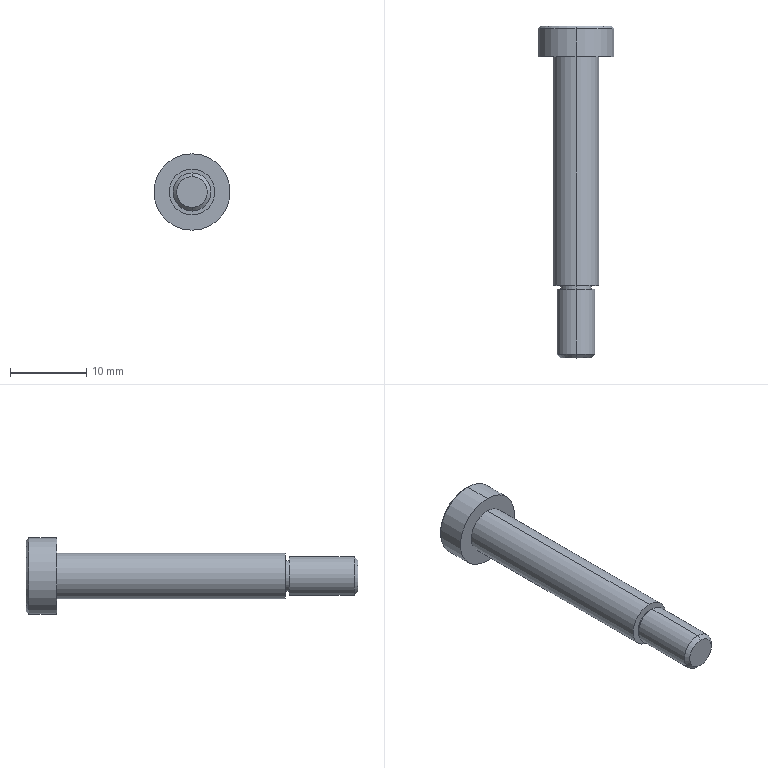Part | SolidWorks | features BaseBody 1, MoveFace 1 | 1 solid | 24 faces | box 10 x 43.5 x 10 mm | volume 1326 mm3 | plane 12 | cylinder 8 | cone 4 | commonest cylinder face diameters 4 x2 5 x2 6 x2 10 x2
STEP:
#1=CARTESIAN_POINT('',(0.,-8.5,3.));
#2=VERTEX_POINT('',#1);
#3=CARTESIAN_POINT('',(0.,-8.5,-3.));
#4=VERTEX_POINT('',#3);
#5=CARTESIAN_POINT('',(0.,-8.5,0.));
#6=DIRECTION('',(0.,1.,0.));
#7=DIRECTION('',(0.,0.,1.));
#8=AXIS2_PLACEMENT_3D('',#5,#6,#7);
#9=CIRCLE('',#8,3.);
#10=EDGE_CURVE('',#2,#4,#9,.T.);
#11=ORIENTED_EDGE('',*,*,#10,.T.);
#12=CARTESIAN_POINT('',(0.,21.5,-3.));
#13=VERTEX_POINT('',#12);
#14=CARTESIAN_POINT('',(0.,0.,-3.));
#15=DIRECTION('',(0.,1.,0.));
#16=VECTOR('',#15,1000.);
#17=LINE('',#14,#16);
#18=EDGE_CURVE('',#4,#13,#17,.T.);
#19=ORIENTED_EDGE('',*,*,#18,.T.);
#20=CARTESIAN_POINT('',(0.,21.5,3.));
#21=VERTEX_POINT('',#20);
#22=CARTESIAN_POINT('',(0.,21.5,0.));
#23=DIRECTION('',(0.,-1.,0.));
#24=DIRECTION('',(0.,0.,1.));
#25=AXIS2_PLACEMENT_3D('',#22,#23,#24);
#26=CIRCLE('',#25,3.);
#27=EDGE_CURVE('',#13,#21,#26,.T.);
#28=ORIENTED_EDGE('',*,*,#27,.T.);
#29=CARTESIAN_POINT('',(0.,0.,3.));
#30=DIRECTION('',(0.,1.,0.));
#31=VECTOR('',#30,1000.);
#32=LINE('',#29,#31);
#33=EDGE_CURVE('',#2,#21,#32,.T.);
#34=ORIENTED_EDGE('',*,*,#33,.F.);
#35=EDGE_LOOP('',(#11,#19,#28,#34));
#36=FACE_OUTER_BOUND('',#35,.T.);
#37=CARTESIAN_POINT('',(0.,0.,0.));
#38=DIRECTION('',(0.,1.,0.));
#39=DIRECTION('',(0.,0.,1.));
#40=AXIS2_PLACEMENT_3D('',#37,#38,#39);
#41=CYLINDRICAL_SURFACE('',#40,3.);
#42=ADVANCED_FACE('',(#36),#41,.T.);
#43=CARTESIAN_POINT('',(0.,21.5,5.));
#44=VERTEX_POINT('',#43);
#45=CARTESIAN_POINT('',(0.,21.5,-5.));
#46=VERTEX_POINT('',#45);
#47=CARTESIAN_POINT('',(0.,21.5,0.));
#48=DIRECTION('',(0.,1.,0.));
#49=DIRECTION('',(0.,0.,1.));
#50=AXIS2_PLACEMENT_3D('',#47,#48,#49);
#51=CIRCLE('',#50,5.);
#52=EDGE_CURVE('',#44,#46,#51,.T.);
#53=ORIENTED_EDGE('',*,*,#52,.T.);
#54=CARTESIAN_POINT('',(0.,25.167,-5.));
#55=VERTEX_POINT('',#54);
#56=CARTESIAN_POINT('',(0.,0.,-5.));
#57=DIRECTION('',(0.,1.,0.));
#58=VECTOR('',#57,1000.);
#59=LINE('',#56,#58);
#60=EDGE_CURVE('',#46,#55,#59,.T.);
#61=ORIENTED_EDGE('',*,*,#60,.T.);
#62=CARTESIAN_POINT('',(0.,25.167,5.));
#63=VERTEX_POINT('',#62);
#64=CARTESIAN_POINT('',(0.,25.167,0.));
#65=DIRECTION('',(0.,-1.,0.));
#66=DIRECTION('',(0.,0.,1.));
#67=AXIS2_PLACEMENT_3D('',#64,#65,#66);
#68=CIRCLE('',#67,5.);
#69=EDGE_CURVE('',#55,#63,#68,.T.);
#70=ORIENTED_EDGE('',*,*,#69,.T.);
#71=CARTESIAN_POINT('',(0.,0.,5.));
#72=DIRECTION('',(0.,1.,0.));
#73=VECTOR('',#72,1000.);
#74=LINE('',#71,#73);
#75=EDGE_CURVE('',#44,#63,#74,.T.);
#76=ORIENTED_EDGE('',*,*,#75,.F.);
#77=EDGE_LOOP('',(#53,#61,#70,#76));
#78=FACE_OUTER_BOUND('',#77,.T.);
#79=CARTESIAN_POINT('',(0.,0.,0.));
#80=DIRECTION('',(0.,1.,0.));
#81=DIRECTION('',(0.,0.,1.));
#82=AXIS2_PLACEMENT_3D('',#79,#80,#81);
#83=CYLINDRICAL_SURFACE('',#82,5.);
#84=ADVANCED_FACE('',(#78),#83,.T.);
#85=CARTESIAN_POINT('',(0.,-9.,2.));
#86=VERTEX_POINT('',#85);
#87=CARTESIAN_POINT('',(0.,-9.,-2.));
#88=VERTEX_POINT('',#87);
#89=CARTESIAN_POINT('',(0.,-9.,0.));
#90=DIRECTION('',(0.,1.,0.));
#91=DIRECTION('',(0.,0.,1.));
#92=AXIS2_PLACEMENT_3D('',#89,#90,#91);
#93=CIRCLE('',#92,2.);
#94=EDGE_CURVE('',#86,#88,#93,.T.);
#95=ORIENTED_EDGE('',*,*,#94,.T.);
#96=CARTESIAN_POINT('',(0.,-8.5,-2.));
#97=VERTEX_POINT('',#96);
#98=CARTESIAN_POINT('',(0.,-18.,-2.));
#99=DIRECTION('',(0.,1.,0.));
#100=VECTOR('',#99,1000.);
#101=LINE('',#98,#100);
#102=EDGE_CURVE('',#88,#97,#101,.T.);
#103=ORIENTED_EDGE('',*,*,#102,.T.);
#104=CARTESIAN_POINT('',(0.,-8.5,2.));
#105=VERTEX_POINT('',#104);
#106=CARTESIAN_POINT('',(0.,-8.5,0.));
#107=DIRECTION('',(0.,-1.,0.));
#108=DIRECTION('',(0.,0.,1.));
#109=AXIS2_PLACEMENT_3D('',#106,#107,#108);
#110=CIRCLE('',#109,2.);
#111=EDGE_CURVE('',#97,#105,#110,.T.);
#112=ORIENTED_EDGE('',*,*,#111,.T.);
#113=CARTESIAN_POINT('',(0.,-18.,2.));
#114=DIRECTION('',(0.,1.,0.));
#115=VECTOR('',#114,1000.);
#116=LINE('',#113,#115);
#117=EDGE_CURVE('',#86,#105,#116,.T.);
#118=ORIENTED_EDGE('',*,*,#117,.F.);
#119=EDGE_LOOP('',(#95,#103,#112,#118));
#120=FACE_OUTER_BOUND('',#119,.T.);
#121=CARTESIAN_POINT('',(0.,-18.,0.));
#122=DIRECTION('',(0.,1.,0.));
#123=DIRECTION('',(0.,0.,1.));
#124=AXIS2_PLACEMENT_3D('',#121,#122,#123);
#125=CYLINDRICAL_SURFACE('',#124,2.);
#126=ADVANCED_FACE('',(#120),#125,.T.);
#127=CARTESIAN_POINT('',(0.,25.5,-4.667));
#128=VERTEX_POINT('',#127);
#129=CARTESIAN_POINT('',(0.,25.5,4.667));
#130=VERTEX_POINT('',#129);
#131=CARTESIAN_POINT('',(0.,25.5,0.));
#132=DIRECTION('',(0.,-1.,0.));
#133=DIRECTION('',(0.,0.,-1.));
#134=AXIS2_PLACEMENT_3D('',#131,#132,#133);
#135=CIRCLE('',#134,4.667);
#136=EDGE_CURVE('',#128,#130,#135,.T.);
#137=ORIENTED_EDGE('',*,*,#136,.T.);
#138=CARTESIAN_POINT('',(0.,25.167,5.));
#139=DIRECTION('',(0.,-0.7071,0.7071));
#140=VECTOR('',#139,1000.);
#141=LINE('',#138,#140);
#142=EDGE_CURVE('',#130,#63,#141,.T.);
#143=ORIENTED_EDGE('',*,*,#142,.T.);
#144=ORIENTED_EDGE('',*,*,#69,.F.);
#145=CARTESIAN_POINT('',(0.,25.167,-5.));
#146=DIRECTION('',(0.,-0.7071,-0.7071));
#147=VECTOR('',#146,1000.);
#148=LINE('',#145,#147);
#149=EDGE_CURVE('',#128,#55,#148,.T.);
#150=ORIENTED_EDGE('',*,*,#149,.F.);
#151=EDGE_LOOP('',(#137,#143,#144,#150));
#152=FACE_OUTER_BOUND('',#151,.T.);
#153=CARTESIAN_POINT('',(0.,25.167,0.));
#154=DIRECTION('',(0.,-1.,0.));
#155=DIRECTION('',(0.,0.,-1.));
#156=AXIS2_PLACEMENT_3D('',#153,#154,#155);
#157=CONICAL_SURFACE('',#156,5.,0.7854);
#158=ADVANCED_FACE('',(#152),#157,.T.);
#159=CARTESIAN_POINT('',(0.,-17.509,2.5));
#160=VERTEX_POINT('',#159);
#161=CARTESIAN_POINT('',(0.,-17.509,-2.5));
#162=VERTEX_POINT('',#161);
#163=CARTESIAN_POINT('',(0.,-17.509,0.));
#164=DIRECTION('',(0.,1.,0.));
#165=DIRECTION('',(0.,0.,1.));
#166=AXIS2_PLACEMENT_3D('',#163,#164,#165);
#167=CIRCLE('',#166,2.5);
#168=EDGE_CURVE('',#160,#162,#167,.T.);
#169=ORIENTED_EDGE('',*,*,#168,.T.);
#170=CARTESIAN_POINT('',(0.,-9.,-2.5));
#171=VERTEX_POINT('',#170);
#172=CARTESIAN_POINT('',(0.,-18.,-2.5));
#173=DIRECTION('',(0.,1.,0.));
#174=VECTOR('',#173,1000.);
#175=LINE('',#172,#174);
#176=EDGE_CURVE('',#162,#171,#175,.T.);
#177=ORIENTED_EDGE('',*,*,#176,.T.);
#178=CARTESIAN_POINT('',(0.,-9.,2.5));
#179=VERTEX_POINT('',#178);
#180=CARTESIAN_POINT('',(0.,-9.,0.));
#181=DIRECTION('',(0.,-1.,0.));
#182=DIRECTION('',(0.,0.,1.));
#183=AXIS2_PLACEMENT_3D('',#180,#181,#182);
#184=CIRCLE('',#183,2.5);
#185=EDGE_CURVE('',#171,#179,#184,.T.);
#186=ORIENTED_EDGE('',*,*,#185,.T.);
#187=CARTESIAN_POINT('',(0.,-18.,2.5));
#188=DIRECTION('',(0.,1.,0.));
#189=VECTOR('',#188,1000.);
#190=LINE('',#187,#189);
#191=EDGE_CURVE('',#160,#179,#190,.T.);
#192=ORIENTED_EDGE('',*,*,#191,.F.);
#193=EDGE_LOOP('',(#169,#177,#186,#192));
#194=FACE_OUTER_BOUND('',#193,.T.);
#195=CARTESIAN_POINT('',(0.,-18.,0.));
#196=DIRECTION('',(0.,1.,0.));
#197=DIRECTION('',(0.,0.,1.));
#198=AXIS2_PLACEMENT_3D('',#195,#196,#197);
#199=CYLINDRICAL_SURFACE('',#198,2.5);
#200=ADVANCED_FACE('',(#194),#199,.T.);
#201=CARTESIAN_POINT('',(0.,-18.,2.009));
#202=VERTEX_POINT('',#201);
#203=CARTESIAN_POINT('',(0.,-18.,-2.009));
#204=VERTEX_POINT('',#203);
#205=CARTESIAN_POINT('',(0.,-18.,0.));
#206=DIRECTION('',(0.,1.,0.));
#207=DIRECTION('',(0.,0.,1.));
#208=AXIS2_PLACEMENT_3D('',#205,#206,#207);
#209=CIRCLE('',#208,2.009);
#210=EDGE_CURVE('',#202,#204,#209,.T.);
#211=ORIENTED_EDGE('',*,*,#210,.T.);
#212=CARTESIAN_POINT('',(0.,-17.509,-2.5));
#213=DIRECTION('',(0.,0.7071,-0.7071));
#214=VECTOR('',#213,1000.);
#215=LINE('',#212,#214);
#216=EDGE_CURVE('',#204,#162,#215,.T.);
#217=ORIENTED_EDGE('',*,*,#216,.T.);
#218=ORIENTED_EDGE('',*,*,#168,.F.);
#219=CARTESIAN_POINT('',(0.,-17.509,2.5));
#220=DIRECTION('',(0.,0.7071,0.7071));
#221=VECTOR('',#220,1000.);
#222=LINE('',#219,#221);
#223=EDGE_CURVE('',#202,#160,#222,.T.);
#224=ORIENTED_EDGE('',*,*,#223,.F.);
#225=EDGE_LOOP('',(#211,#217,#218,#224));
#226=FACE_OUTER_BOUND('',#225,.T.);
#227=CARTESIAN_POINT('',(0.,-17.509,0.));
#228=DIRECTION('',(0.,1.,0.));
#229=DIRECTION('',(0.,0.,1.));
#230=AXIS2_PLACEMENT_3D('',#227,#228,#229);
#231=CONICAL_SURFACE('',#230,2.5,0.7854);
#232=ADVANCED_FACE('',(#226),#231,.T.);
#233=ORIENTED_EDGE('',*,*,#18,.F.);
#234=CARTESIAN_POINT('',(0.,-8.5,0.));
#235=DIRECTION('',(0.,1.,0.));
#236=DIRECTION('',(0.,0.,1.));
#237=AXIS2_PLACEMENT_3D('',#234,#235,#236);
#238=CIRCLE('',#237,3.);
#239=EDGE_CURVE('',#4,#2,#238,.T.);
#240=ORIENTED_EDGE('',*,*,#239,.T.);
#241=ORIENTED_EDGE('',*,*,#33,.T.);
#242=CARTESIAN_POINT('',(0.,21.5,0.));
#243=DIRECTION('',(0.,-1.,0.));
#244=DIRECTION('',(0.,0.,1.));
#245=AXIS2_PLACEMENT_3D('',#242,#243,#244);
#246=CIRCLE('',#245,3.);
#247=EDGE_CURVE('',#21,#13,#246,.T.);
#248=ORIENTED_EDGE('',*,*,#247,.T.);
#249=EDGE_LOOP('',(#233,#240,#241,#248));
#250=FACE_OUTER_BOUND('',#249,.T.);
#251=CARTESIAN_POINT('',(0.,0.,0.));
#252=DIRECTION('',(0.,1.,0.));
#253=DIRECTION('',(0.,0.,1.));
#254=AXIS2_PLACEMENT_3D('',#251,#252,#253);
#255=CYLINDRICAL_SURFACE('',#254,3.);
#256=ADVANCED_FACE('',(#250),#255,.T.);
#257=ORIENTED_EDGE('',*,*,#52,.F.);
#258=CARTESIAN_POINT('',(0.,21.5,0.));
#259=DIRECTION('',(0.,1.,0.));
#260=DIRECTION('',(0.,0.,1.));
#261=AXIS2_PLACEMENT_3D('',#258,#259,#260);
#262=CIRCLE('',#261,5.);
#263=EDGE_CURVE('',#46,#44,#262,.T.);
#264=ORIENTED_EDGE('',*,*,#263,.F.);
#265=EDGE_LOOP('',(#257,#264));
#266=FACE_OUTER_BOUND('',#265,.T.);
#267=ORIENTED_EDGE('',*,*,#247,.F.);
#268=ORIENTED_EDGE('',*,*,#27,.F.);
#269=EDGE_LOOP('',(#267,#268));
#270=FACE_BOUND('',#269,.T.);
#271=CARTESIAN_POINT('',(5.,21.5,0.));
#272=DIRECTION('',(0.,1.,0.));
#273=DIRECTION('',(0.,0.,1.));
#274=AXIS2_PLACEMENT_3D('',#271,#272,#273);
#275=PLANE('',#274);
#276=ADVANCED_FACE('',(#266,#270),#275,.F.);
#277=ORIENTED_EDGE('',*,*,#10,.F.);
#278=ORIENTED_EDGE('',*,*,#239,.F.);
#279=EDGE_LOOP('',(#277,#278));
#280=FACE_OUTER_BOUND('',#279,.T.);
#281=CARTESIAN_POINT('',(0.,-8.5,0.));
#282=DIRECTION('',(0.,-1.,0.));
#283=DIRECTION('',(0.,0.,1.));
#284=AXIS2_PLACEMENT_3D('',#281,#282,#283);
#285=CIRCLE('',#284,2.);
#286=EDGE_CURVE('',#105,#97,#285,.T.);
#287=ORIENTED_EDGE('',*,*,#286,.F.);
#288=ORIENTED_EDGE('',*,*,#111,.F.);
#289=EDGE_LOOP('',(#287,#288));
#290=FACE_BOUND('',#289,.T.);
#291=CARTESIAN_POINT('',(3.,-8.5,0.));
#292=DIRECTION('',(0.,1.,0.));
#293=DIRECTION('',(0.,0.,1.));
#294=AXIS2_PLACEMENT_3D('',#291,#292,#293);
#295=PLANE('',#294);
#296=ADVANCED_FACE('',(#280,#290),#295,.F.);
#297=ORIENTED_EDGE('',*,*,#60,.F.);
#298=ORIENTED_EDGE('',*,*,#263,.T.);
#299=ORIENTED_EDGE('',*,*,#75,.T.);
#300=CARTESIAN_POINT('',(0.,25.167,0.));
#301=DIRECTION('',(0.,-1.,0.));
#302=DIRECTION('',(0.,0.,1.));
#303=AXIS2_PLACEMENT_3D('',#300,#301,#302);
#304=CIRCLE('',#303,5.);
#305=EDGE_CURVE('',#63,#55,#304,.T.);
#306=ORIENTED_EDGE('',*,*,#305,.T.);
#307=EDGE_LOOP('',(#297,#298,#299,#306));
#308=FACE_OUTER_BOUND('',#307,.T.);
#309=CARTESIAN_POINT('',(0.,0.,0.));
#310=DIRECTION('',(0.,1.,0.));
#311=DIRECTION('',(0.,0.,1.));
#312=AXIS2_PLACEMENT_3D('',#309,#310,#311);
#313=CYLINDRICAL_SURFACE('',#312,5.);
#314=ADVANCED_FACE('',(#308),#313,.T.);
#315=ORIENTED_EDGE('',*,*,#102,.F.);
#316=CARTESIAN_POINT('',(0.,-9.,0.));
#317=DIRECTION('',(0.,1.,0.));
#318=DIRECTION('',(0.,0.,1.));
#319=AXIS2_PLACEMENT_3D('',#316,#317,#318);
#320=CIRCLE('',#319,2.);
#321=EDGE_CURVE('',#88,#86,#320,.T.);
#322=ORIENTED_EDGE('',*,*,#321,.T.);
#323=ORIENTED_EDGE('',*,*,#117,.T.);
#324=ORIENTED_EDGE('',*,*,#286,.T.);
#325=EDGE_LOOP('',(#315,#322,#323,#324));
#326=FACE_OUTER_BOUND('',#325,.T.);
#327=CARTESIAN_POINT('',(0.,-18.,0.));
#328=DIRECTION('',(0.,1.,0.));
#329=DIRECTION('',(0.,0.,1.));
#330=AXIS2_PLACEMENT_3D('',#327,#328,#329);
#331=CYLINDRICAL_SURFACE('',#330,2.);
#332=ADVANCED_FACE('',(#326),#331,.T.);
#333=ORIENTED_EDGE('',*,*,#142,.F.);
#334=CARTESIAN_POINT('',(0.,25.5,0.));
#335=DIRECTION('',(0.,-1.,0.));
#336=DIRECTION('',(0.,0.,-1.));
#337=AXIS2_PLACEMENT_3D('',#334,#335,#336);
#338=CIRCLE('',#337,4.667);
#339=EDGE_CURVE('',#130,#128,#338,.T.);
#340=ORIENTED_EDGE('',*,*,#339,.T.);
#341=ORIENTED_EDGE('',*,*,#149,.T.);
#342=ORIENTED_EDGE('',*,*,#305,.F.);
#343=EDGE_LOOP('',(#333,#340,#341,#342));
#344=FACE_OUTER_BOUND('',#343,.T.);
#345=CARTESIAN_POINT('',(0.,25.167,0.));
#346=DIRECTION('',(0.,-1.,0.));
#347=DIRECTION('',(0.,0.,-1.));
#348=AXIS2_PLACEMENT_3D('',#345,#346,#347);
#349=CONICAL_SURFACE('',#348,5.,0.7854);
#350=ADVANCED_FACE('',(#344),#349,.T.);
#351=ORIENTED_EDGE('',*,*,#94,.F.);
#352=ORIENTED_EDGE('',*,*,#321,.F.);
#353=EDGE_LOOP('',(#351,#352));
#354=FACE_BOUND('',#353,.T.);
#355=CARTESIAN_POINT('',(0.,-9.,0.));
#356=DIRECTION('',(0.,-1.,0.));
#357=DIRECTION('',(0.,0.,1.));
#358=AXIS2_PLACEMENT_3D('',#355,#356,#357);
#359=CIRCLE('',#358,2.5);
#360=EDGE_CURVE('',#179,#171,#359,.T.);
#361=ORIENTED_EDGE('',*,*,#360,.F.);
#362=ORIENTED_EDGE('',*,*,#185,.F.);
#363=EDGE_LOOP('',(#361,#362));
#364=FACE_OUTER_BOUND('',#363,.T.);
#365=CARTESIAN_POINT('',(2.,-9.,0.));
#366=DIRECTION('',(0.,-1.,0.));
#367=DIRECTION('',(0.,0.,-1.));
#368=AXIS2_PLACEMENT_3D('',#365,#366,#367);
#369=PLANE('',#368);
#370=ADVANCED_FACE('',(#354,#364),#369,.F.);
#371=CARTESIAN_POINT('',(0.,25.5,1.732));
#372=VERTEX_POINT('',#371);
#373=CARTESIAN_POINT('',(-1.5,25.5,0.866));
#374=VERTEX_POINT('',#373);
#375=CARTESIAN_POINT('',(-1.5,25.5,0.866));
#376=DIRECTION('',(-0.866,0.,-0.5));
#377=VECTOR('',#376,1000.);
#378=LINE('',#375,#377);
#379=EDGE_CURVE('',#372,#374,#378,.T.);
#380=ORIENTED_EDGE('',*,*,#379,.T.);
#381=CARTESIAN_POINT('',(-1.5,25.5,-0.866));
#382=VERTEX_POINT('',#381);
#383=CARTESIAN_POINT('',(-1.5,25.5,-0.866));
#384=DIRECTION('',(0.,0.,-1.));
#385=VECTOR('',#384,1000.);
#386=LINE('',#383,#385);
#387=EDGE_CURVE('',#374,#382,#386,.T.);
#388=ORIENTED_EDGE('',*,*,#387,.T.);
#389=CARTESIAN_POINT('',(0.,25.5,-1.732));
#390=VERTEX_POINT('',#389);
#391=CARTESIAN_POINT('',(0.,25.5,-1.732));
#392=DIRECTION('',(0.866,0.,-0.5));
#393=VECTOR('',#392,1000.);
#394=LINE('',#391,#393);
#395=EDGE_CURVE('',#382,#390,#394,.T.);
#396=ORIENTED_EDGE('',*,*,#395,.T.);
#397=CARTESIAN_POINT('',(1.5,25.5,-0.866));
#398=VERTEX_POINT('',#397);
#399=CARTESIAN_POINT('',(1.5,25.5,-0.866));
#400=DIRECTION('',(0.866,0.,0.5));
#401=VECTOR('',#400,1000.);
#402=LINE('',#399,#401);
#403=EDGE_CURVE('',#390,#398,#402,.T.);
#404=ORIENTED_EDGE('',*,*,#403,.T.);
#405=CARTESIAN_POINT('',(1.5,25.5,0.866));
#406=VERTEX_POINT('',#405);
#407=CARTESIAN_POINT('',(1.5,25.5,0.866));
#408=DIRECTION('',(0.,0.,1.));
#409=VECTOR('',#408,1000.);
#410=LINE('',#407,#409);
#411=EDGE_CURVE('',#398,#406,#410,.T.);
#412=ORIENTED_EDGE('',*,*,#411,.T.);
#413=CARTESIAN_POINT('',(0.,25.5,1.732));
#414=DIRECTION('',(0.866,0.,-0.5));
#415=VECTOR('',#414,1000.);
#416=LINE('',#413,#415);
#417=EDGE_CURVE('',#372,#406,#416,.T.);
#418=ORIENTED_EDGE('',*,*,#417,.F.);
#419=EDGE_LOOP('',(#380,#388,#396,#404,#412,#418));
#420=FACE_BOUND('',#419,.T.);
#421=ORIENTED_EDGE('',*,*,#136,.F.);
#422=ORIENTED_EDGE('',*,*,#339,.F.);
#423=EDGE_LOOP('',(#421,#422));
#424=FACE_OUTER_BOUND('',#423,.T.);
#425=CARTESIAN_POINT('',(0.,25.5,0.));
#426=DIRECTION('',(0.,-1.,0.));
#427=DIRECTION('',(0.,0.,-1.));
#428=AXIS2_PLACEMENT_3D('',#425,#426,#427);
#429=PLANE('',#428);
#430=ADVANCED_FACE('',(#420,#424),#429,.F.);
#431=ORIENTED_EDGE('',*,*,#176,.F.);
#432=CARTESIAN_POINT('',(0.,-17.509,0.));
#433=DIRECTION('',(0.,1.,0.));
#434=DIRECTION('',(0.,0.,1.));
#435=AXIS2_PLACEMENT_3D('',#432,#433,#434);
#436=CIRCLE('',#435,2.5);
#437=EDGE_CURVE('',#162,#160,#436,.T.);
#438=ORIENTED_EDGE('',*,*,#437,.T.);
#439=ORIENTED_EDGE('',*,*,#191,.T.);
#440=ORIENTED_EDGE('',*,*,#360,.T.);
#441=EDGE_LOOP('',(#431,#438,#439,#440));
#442=FACE_OUTER_BOUND('',#441,.T.);
#443=CARTESIAN_POINT('',(0.,-18.,0.));
#444=DIRECTION('',(0.,1.,0.));
#445=DIRECTION('',(0.,0.,1.));
#446=AXIS2_PLACEMENT_3D('',#443,#444,#445);
#447=CYLINDRICAL_SURFACE('',#446,2.5);
#448=ADVANCED_FACE('',(#442),#447,.T.);
#449=CARTESIAN_POINT('',(1.5,23.5,0.866));
#450=VERTEX_POINT('',#449);
#451=CARTESIAN_POINT('',(1.5,23.5,0.866));
#452=DIRECTION('',(0.,1.,0.));
#453=VECTOR('',#452,1000.);
#454=LINE('',#451,#453);
#455=EDGE_CURVE('',#450,#406,#454,.T.);
#456=ORIENTED_EDGE('',*,*,#455,.F.);
#457=CARTESIAN_POINT('',(0.,23.5,1.732));
#458=VERTEX_POINT('',#457);
#459=CARTESIAN_POINT('',(0.,23.5,1.732));
#460=DIRECTION('',(0.866,0.,-0.5));
#461=VECTOR('',#460,1000.);
#462=LINE('',#459,#461);
#463=EDGE_CURVE('',#458,#450,#462,.T.);
#464=ORIENTED_EDGE('',*,*,#463,.F.);
#465=CARTESIAN_POINT('',(0.,23.5,1.732));
#466=DIRECTION('',(0.,-1.,0.));
#467=VECTOR('',#466,1000.);
#468=LINE('',#465,#467);
#469=EDGE_CURVE('',#372,#458,#468,.T.);
#470=ORIENTED_EDGE('',*,*,#469,.F.);
#471=ORIENTED_EDGE('',*,*,#417,.T.);
#472=EDGE_LOOP('',(#456,#464,#470,#471));
#473=FACE_OUTER_BOUND('',#472,.T.);
#474=CARTESIAN_POINT('',(0.,23.5,1.732));
#475=DIRECTION('',(0.5,0.,0.866));
#476=DIRECTION('',(0.866,0.,-0.5));
#477=AXIS2_PLACEMENT_3D('',#474,#475,#476);
#478=PLANE('',#477);
#479=ADVANCED_FACE('',(#473),#478,.F.);
#480=ORIENTED_EDGE('',*,*,#216,.F.);
#481=CARTESIAN_POINT('',(0.,-18.,0.));
#482=DIRECTION('',(0.,1.,0.));
#483=DIRECTION('',(0.,0.,1.));
#484=AXIS2_PLACEMENT_3D('',#481,#482,#483);
#485=CIRCLE('',#484,2.009);
#486=EDGE_CURVE('',#204,#202,#485,.T.);
#487=ORIENTED_EDGE('',*,*,#486,.T.);
#488=ORIENTED_EDGE('',*,*,#223,.T.);
#489=ORIENTED_EDGE('',*,*,#437,.F.);
#490=EDGE_LOOP('',(#480,#487,#488,#489));
#491=FACE_OUTER_BOUND('',#490,.T.);
#492=CARTESIAN_POINT('',(0.,-17.509,0.));
#493=DIRECTION('',(0.,1.,0.));
#494=DIRECTION('',(0.,0.,1.));
#495=AXIS2_PLACEMENT_3D('',#492,#493,#494);
#496=CONICAL_SURFACE('',#495,2.5,0.7854);
#497=ADVANCED_FACE('',(#491),#496,.T.);
#498=ORIENTED_EDGE('',*,*,#411,.F.);
#499=CARTESIAN_POINT('',(1.5,23.5,-0.866));
#500=VERTEX_POINT('',#499);
#501=CARTESIAN_POINT('',(1.5,23.5,-0.866));
#502=DIRECTION('',(0.,1.,0.));
#503=VECTOR('',#502,1000.);
#504=LINE('',#501,#503);
#505=EDGE_CURVE('',#500,#398,#504,.T.);
#506=ORIENTED_EDGE('',*,*,#505,.F.);
#507=CARTESIAN_POINT('',(1.5,23.5,0.866));
#508=DIRECTION('',(0.,0.,-1.));
#509=VECTOR('',#508,1000.);
#510=LINE('',#507,#509);
#511=EDGE_CURVE('',#450,#500,#510,.T.);
#512=ORIENTED_EDGE('',*,*,#511,.F.);
#513=ORIENTED_EDGE('',*,*,#455,.T.);
#514=EDGE_LOOP('',(#498,#506,#512,#513));
#515=FACE_OUTER_BOUND('',#514,.T.);
#516=CARTESIAN_POINT('',(1.5,23.5,0.866));
#517=DIRECTION('',(1.,0.,0.));
#518=DIRECTION('',(0.,0.,-1.));
#519=AXIS2_PLACEMENT_3D('',#516,#517,#518);
#520=PLANE('',#519);
#521=ADVANCED_FACE('',(#515),#520,.F.);
#522=CARTESIAN_POINT('',(0.,23.5,-1.732));
#523=VERTEX_POINT('',#522);
#524=CARTESIAN_POINT('',(1.5,23.5,-0.866));
#525=DIRECTION('',(-0.866,0.,-0.5));
#526=VECTOR('',#525,1000.);
#527=LINE('',#524,#526);
#528=EDGE_CURVE('',#500,#523,#527,.T.);
#529=ORIENTED_EDGE('',*,*,#528,.T.);
#530=CARTESIAN_POINT('',(-1.5,23.5,-0.866));
#531=VERTEX_POINT('',#530);
#532=CARTESIAN_POINT('',(0.,23.5,-1.732));
#533=DIRECTION('',(-0.866,0.,0.5));
#534=VECTOR('',#533,1000.);
#535=LINE('',#532,#534);
#536=EDGE_CURVE('',#523,#531,#535,.T.);
#537=ORIENTED_EDGE('',*,*,#536,.T.);
#538=CARTESIAN_POINT('',(-1.5,23.5,0.866));
#539=VERTEX_POINT('',#538);
#540=CARTESIAN_POINT('',(-1.5,23.5,-0.866));
#541=DIRECTION('',(0.,0.,1.));
#542=VECTOR('',#541,1000.);
#543=LINE('',#540,#542);
#544=EDGE_CURVE('',#531,#539,#543,.T.);
#545=ORIENTED_EDGE('',*,*,#544,.T.);
#546=CARTESIAN_POINT('',(-1.5,23.5,0.866));
#547=DIRECTION('',(0.866,0.,0.5));
#548=VECTOR('',#547,1000.);
#549=LINE('',#546,#548);
#550=EDGE_CURVE('',#539,#458,#549,.T.);
#551=ORIENTED_EDGE('',*,*,#550,.T.);
#552=ORIENTED_EDGE('',*,*,#463,.T.);
#553=ORIENTED_EDGE('',*,*,#511,.T.);
#554=EDGE_LOOP('',(#529,#537,#545,#551,#552,#553));
#555=FACE_OUTER_BOUND('',#554,.T.);
#556=CARTESIAN_POINT('',(0.,23.5,0.));
#557=DIRECTION('',(0.,1.,0.));
#558=DIRECTION('',(0.,0.,1.));
#559=AXIS2_PLACEMENT_3D('',#556,#557,#558);
#560=PLANE('',#559);
#561=ADVANCED_FACE('',(#555),#560,.T.);
#562=ORIENTED_EDGE('',*,*,#469,.T.);
#563=ORIENTED_EDGE('',*,*,#550,.F.);
#564=CARTESIAN_POINT('',(-1.5,23.5,0.866));
#565=DIRECTION('',(0.,-1.,0.));
#566=VECTOR('',#565,1000.);
#567=LINE('',#564,#566);
#568=EDGE_CURVE('',#374,#539,#567,.T.);
#569=ORIENTED_EDGE('',*,*,#568,.F.);
#570=ORIENTED_EDGE('',*,*,#379,.F.);
#571=EDGE_LOOP('',(#562,#563,#569,#570));
#572=FACE_OUTER_BOUND('',#571,.T.);
#573=CARTESIAN_POINT('',(-1.5,23.5,0.866));
#574=DIRECTION('',(-0.5,0.,0.866));
#575=DIRECTION('',(0.866,0.,0.5));
#576=AXIS2_PLACEMENT_3D('',#573,#574,#575);
#577=PLANE('',#576);
#578=ADVANCED_FACE('',(#572),#577,.F.);
#579=ORIENTED_EDGE('',*,*,#210,.F.);
#580=ORIENTED_EDGE('',*,*,#486,.F.);
#581=EDGE_LOOP('',(#579,#580));
#582=FACE_OUTER_BOUND('',#581,.T.);
#583=CARTESIAN_POINT('',(2.01,-18.,0.));
#584=DIRECTION('',(0.,1.,0.));
#585=DIRECTION('',(0.,0.,1.));
#586=AXIS2_PLACEMENT_3D('',#583,#584,#585);
#587=PLANE('',#586);
#588=ADVANCED_FACE('',(#582),#587,.F.);
#589=CARTESIAN_POINT('',(0.,23.5,-1.732));
#590=DIRECTION('',(0.,1.,0.));
#591=VECTOR('',#590,1000.);
#592=LINE('',#589,#591);
#593=EDGE_CURVE('',#523,#390,#592,.T.);
#594=ORIENTED_EDGE('',*,*,#593,.F.);
#595=ORIENTED_EDGE('',*,*,#528,.F.);
#596=ORIENTED_EDGE('',*,*,#505,.T.);
#597=ORIENTED_EDGE('',*,*,#403,.F.);
#598=EDGE_LOOP('',(#594,#595,#596,#597));
#599=FACE_OUTER_BOUND('',#598,.T.);
#600=CARTESIAN_POINT('',(1.5,23.5,-0.866));
#601=DIRECTION('',(0.5,0.,-0.866));
#602=DIRECTION('',(-0.866,0.,-0.5));
#603=AXIS2_PLACEMENT_3D('',#600,#601,#602);
#604=PLANE('',#603);
#605=ADVANCED_FACE('',(#599),#604,.F.);
#606=ORIENTED_EDGE('',*,*,#568,.T.);
#607=ORIENTED_EDGE('',*,*,#544,.F.);
#608=CARTESIAN_POINT('',(-1.5,23.5,-0.866));
#609=DIRECTION('',(0.,-1.,0.));
#610=VECTOR('',#609,1000.);
#611=LINE('',#608,#610);
#612=EDGE_CURVE('',#382,#531,#611,.T.);
#613=ORIENTED_EDGE('',*,*,#612,.F.);
#614=ORIENTED_EDGE('',*,*,#387,.F.);
#615=EDGE_LOOP('',(#606,#607,#613,#614));
#616=FACE_OUTER_BOUND('',#615,.T.);
#617=CARTESIAN_POINT('',(-1.5,23.5,-0.866));
#618=DIRECTION('',(-1.,0.,0.));
#619=DIRECTION('',(0.,0.,1.));
#620=AXIS2_PLACEMENT_3D('',#617,#618,#619);
#621=PLANE('',#620);
#622=ADVANCED_FACE('',(#616),#621,.F.);
#623=ORIENTED_EDGE('',*,*,#612,.T.);
#624=ORIENTED_EDGE('',*,*,#536,.F.);
#625=ORIENTED_EDGE('',*,*,#593,.T.);
#626=ORIENTED_EDGE('',*,*,#395,.F.);
#627=EDGE_LOOP('',(#623,#624,#625,#626));
#628=FACE_OUTER_BOUND('',#627,.T.);
#629=CARTESIAN_POINT('',(0.,23.5,-1.732));
#630=DIRECTION('',(-0.5,0.,-0.866));
#631=DIRECTION('',(-0.866,0.,0.5));
#632=AXIS2_PLACEMENT_3D('',#629,#630,#631);
#633=PLANE('',#632);
#634=ADVANCED_FACE('',(#628),#633,.F.);
#635=CLOSED_SHELL('',(#42,#84,#126,#158,#200,#232,#256,#276,#296,#314,#332,#350,#370,#430,#448,#479,#497,#521,#561,#578,#588,#605,#622,#634));
#636=MANIFOLD_SOLID_BREP('',#635);
#637=CARTESIAN_POINT('',(0.,0.,0.));
#638=DIRECTION('',(0.,0.,1.));
#639=DIRECTION('',(1.,0.,0.));
#640=AXIS2_PLACEMENT_3D('',#637,#638,#639);
#641=(LENGTH_UNIT()NAMED_UNIT(*)SI_UNIT(.MILLI.,.METRE.));
#642=UNCERTAINTY_MEASURE_WITH_UNIT(LENGTH_MEASURE(0.00001),#641,'','');
#643=(NAMED_UNIT(*)PLANE_ANGLE_UNIT()SI_UNIT($,.RADIAN.));
#644=(NAMED_UNIT(*)SI_UNIT($,.STERADIAN.)SOLID_ANGLE_UNIT());
#645=(GEOMETRIC_REPRESENTATION_CONTEXT(3)GLOBAL_UNCERTAINTY_ASSIGNED_CONTEXT((#642))GLOBAL_UNIT_ASSIGNED_CONTEXT((#641,#643,#644))REPRESENTATION_CONTEXT('',''));
#646=ADVANCED_BREP_SHAPE_REPRESENTATION('',(#636,#640),#645);